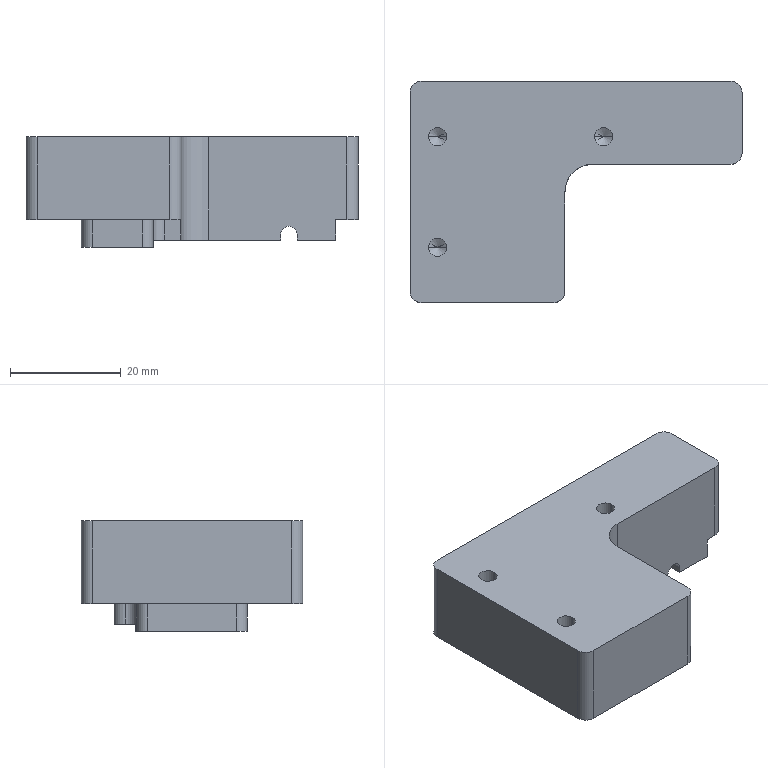Part | STEP file | 05-07 pre-press block | 1 solid | 48 faces | box 60 x 40 x 20 mm | volume 26248 mm3 | cylinder 21 | plane 21 | cone 6 | commonest cylinder face diameters 4 x12 3.3 x6 3 x2 10 x1
STEP:
#1=CARTESIAN_POINT('',(27.5,5.,3.8));
#2=VERTEX_POINT('',#1);
#3=CARTESIAN_POINT('',(29.,5.,2.3));
#4=VERTEX_POINT('',#3);
#5=CARTESIAN_POINT('',(27.5,5.,2.3));
#6=DIRECTION('',(0.,1.,0.));
#7=DIRECTION('',(-1.,0.,0.));
#8=AXIS2_PLACEMENT_3D('',#5,#6,#7);
#9=CIRCLE('',#8,1.5);
#10=EDGE_CURVE('',#2,#4,#9,.T.);
#11=ORIENTED_EDGE('',*,*,#10,.F.);
#12=CARTESIAN_POINT('',(27.5,14.096,3.8));
#13=VERTEX_POINT('',#12);
#14=CARTESIAN_POINT('',(27.5,4.096,3.8));
#15=DIRECTION('',(0.,1.,0.));
#16=VECTOR('',#15,1000.);
#17=LINE('',#14,#16);
#18=EDGE_CURVE('',#2,#13,#17,.T.);
#19=ORIENTED_EDGE('',*,*,#18,.T.);
#20=CARTESIAN_POINT('',(29.,14.096,2.3));
#21=VERTEX_POINT('',#20);
#22=CARTESIAN_POINT('',(27.5,14.096,2.3));
#23=DIRECTION('',(0.,1.,0.));
#24=DIRECTION('',(0.,0.,1.));
#25=AXIS2_PLACEMENT_3D('',#22,#23,#24);
#26=CIRCLE('',#25,1.5);
#27=EDGE_CURVE('',#13,#21,#26,.T.);
#28=ORIENTED_EDGE('',*,*,#27,.T.);
#29=CARTESIAN_POINT('',(29.,4.096,2.3));
#30=DIRECTION('',(0.,1.,0.));
#31=VECTOR('',#30,1000.);
#32=LINE('',#29,#31);
#33=EDGE_CURVE('',#4,#21,#32,.T.);
#34=ORIENTED_EDGE('',*,*,#33,.F.);
#35=EDGE_LOOP('',(#11,#19,#28,#34));
#36=FACE_OUTER_BOUND('',#35,.T.);
#37=CARTESIAN_POINT('',(27.5,4.096,2.3));
#38=DIRECTION('',(0.,1.,0.));
#39=DIRECTION('',(0.,0.,1.));
#40=AXIS2_PLACEMENT_3D('',#37,#38,#39);
#41=CYLINDRICAL_SURFACE('',#40,1.5);
#42=ADVANCED_FACE('',(#36),#41,.F.);
#43=CARTESIAN_POINT('',(-16.65,-10.,8.5));
#44=VERTEX_POINT('',#43);
#45=CARTESIAN_POINT('',(-13.35,-10.,8.5));
#46=VERTEX_POINT('',#45);
#47=CARTESIAN_POINT('',(-15.,-10.,8.5));
#48=DIRECTION('',(0.,0.,1.));
#49=DIRECTION('',(1.,0.,0.));
#50=AXIS2_PLACEMENT_3D('',#47,#48,#49);
#51=CIRCLE('',#50,1.65);
#52=EDGE_CURVE('',#44,#46,#51,.T.);
#53=ORIENTED_EDGE('',*,*,#52,.F.);
#54=CARTESIAN_POINT('',(-16.65,-10.,20.));
#55=VERTEX_POINT('',#54);
#56=CARTESIAN_POINT('',(-16.65,-10.,20.));
#57=DIRECTION('',(0.,0.,1.));
#58=VECTOR('',#57,1000.);
#59=LINE('',#56,#58);
#60=EDGE_CURVE('',#44,#55,#59,.T.);
#61=ORIENTED_EDGE('',*,*,#60,.T.);
#62=CARTESIAN_POINT('',(-13.35,-10.,20.));
#63=VERTEX_POINT('',#62);
#64=CARTESIAN_POINT('',(-15.,-10.,20.));
#65=DIRECTION('',(0.,0.,1.));
#66=DIRECTION('',(1.,0.,0.));
#67=AXIS2_PLACEMENT_3D('',#64,#65,#66);
#68=CIRCLE('',#67,1.65);
#69=EDGE_CURVE('',#55,#63,#68,.T.);
#70=ORIENTED_EDGE('',*,*,#69,.T.);
#71=CARTESIAN_POINT('',(-13.35,-10.,20.));
#72=DIRECTION('',(0.,0.,1.));
#73=VECTOR('',#72,1000.);
#74=LINE('',#71,#73);
#75=EDGE_CURVE('',#46,#63,#74,.T.);
#76=ORIENTED_EDGE('',*,*,#75,.F.);
#77=EDGE_LOOP('',(#53,#61,#70,#76));
#78=FACE_OUTER_BOUND('',#77,.T.);
#79=CARTESIAN_POINT('',(-15.,-10.,20.));
#80=DIRECTION('',(0.,0.,1.));
#81=DIRECTION('',(1.,0.,0.));
#82=AXIS2_PLACEMENT_3D('',#79,#80,#81);
#83=CYLINDRICAL_SURFACE('',#82,1.65);
#84=ADVANCED_FACE('',(#78),#83,.F.);
#85=CARTESIAN_POINT('',(-15.,-10.,7.509));
#86=VERTEX_POINT('',#85);
#87=CARTESIAN_POINT('',(-13.35,-10.,8.5));
#88=DIRECTION('',(0.8572,0.,0.515));
#89=VECTOR('',#88,1000.);
#90=LINE('',#87,#89);
#91=EDGE_CURVE('',#86,#46,#90,.T.);
#92=ORIENTED_EDGE('',*,*,#91,.F.);
#93=CARTESIAN_POINT('',(-16.65,-10.,8.5));
#94=DIRECTION('',(-0.8572,0.,0.515));
#95=VECTOR('',#94,1000.);
#96=LINE('',#93,#95);
#97=EDGE_CURVE('',#86,#44,#96,.T.);
#98=ORIENTED_EDGE('',*,*,#97,.T.);
#99=ORIENTED_EDGE('',*,*,#52,.T.);
#100=EDGE_LOOP('',(#92,#98,#99));
#101=FACE_OUTER_BOUND('',#100,.T.);
#102=CARTESIAN_POINT('',(-15.,-10.,8.5));
#103=DIRECTION('',(0.,0.,1.));
#104=DIRECTION('',(1.,0.,0.));
#105=AXIS2_PLACEMENT_3D('',#102,#103,#104);
#106=CONICAL_SURFACE('',#105,1.65,1.03);
#107=ADVANCED_FACE('',(#101),#106,.F.);
#108=CARTESIAN_POINT('',(13.35,10.,8.5));
#109=VERTEX_POINT('',#108);
#110=CARTESIAN_POINT('',(16.65,10.,8.5));
#111=VERTEX_POINT('',#110);
#112=CARTESIAN_POINT('',(15.,10.,8.5));
#113=DIRECTION('',(0.,0.,1.));
#114=DIRECTION('',(1.,0.,0.));
#115=AXIS2_PLACEMENT_3D('',#112,#113,#114);
#116=CIRCLE('',#115,1.65);
#117=EDGE_CURVE('',#109,#111,#116,.T.);
#118=ORIENTED_EDGE('',*,*,#117,.F.);
#119=CARTESIAN_POINT('',(13.35,10.,20.));
#120=VERTEX_POINT('',#119);
#121=CARTESIAN_POINT('',(13.35,10.,20.));
#122=DIRECTION('',(0.,0.,1.));
#123=VECTOR('',#122,1000.);
#124=LINE('',#121,#123);
#125=EDGE_CURVE('',#109,#120,#124,.T.);
#126=ORIENTED_EDGE('',*,*,#125,.T.);
#127=CARTESIAN_POINT('',(16.65,10.,20.));
#128=VERTEX_POINT('',#127);
#129=CARTESIAN_POINT('',(15.,10.,20.));
#130=DIRECTION('',(0.,0.,1.));
#131=DIRECTION('',(1.,0.,0.));
#132=AXIS2_PLACEMENT_3D('',#129,#130,#131);
#133=CIRCLE('',#132,1.65);
#134=EDGE_CURVE('',#120,#128,#133,.T.);
#135=ORIENTED_EDGE('',*,*,#134,.T.);
#136=CARTESIAN_POINT('',(16.65,10.,20.));
#137=DIRECTION('',(0.,0.,1.));
#138=VECTOR('',#137,1000.);
#139=LINE('',#136,#138);
#140=EDGE_CURVE('',#111,#128,#139,.T.);
#141=ORIENTED_EDGE('',*,*,#140,.F.);
#142=EDGE_LOOP('',(#118,#126,#135,#141));
#143=FACE_OUTER_BOUND('',#142,.T.);
#144=CARTESIAN_POINT('',(15.,10.,20.));
#145=DIRECTION('',(0.,0.,1.));
#146=DIRECTION('',(1.,0.,0.));
#147=AXIS2_PLACEMENT_3D('',#144,#145,#146);
#148=CYLINDRICAL_SURFACE('',#147,1.65);
#149=ADVANCED_FACE('',(#143),#148,.F.);
#150=CARTESIAN_POINT('',(15.,10.,7.509));
#151=VERTEX_POINT('',#150);
#152=CARTESIAN_POINT('',(16.65,10.,8.5));
#153=DIRECTION('',(0.8572,0.,0.515));
#154=VECTOR('',#153,1000.);
#155=LINE('',#152,#154);
#156=EDGE_CURVE('',#151,#111,#155,.T.);
#157=ORIENTED_EDGE('',*,*,#156,.F.);
#158=CARTESIAN_POINT('',(13.35,10.,8.5));
#159=DIRECTION('',(-0.8572,0.,0.515));
#160=VECTOR('',#159,1000.);
#161=LINE('',#158,#160);
#162=EDGE_CURVE('',#151,#109,#161,.T.);
#163=ORIENTED_EDGE('',*,*,#162,.T.);
#164=ORIENTED_EDGE('',*,*,#117,.T.);
#165=EDGE_LOOP('',(#157,#163,#164));
#166=FACE_OUTER_BOUND('',#165,.T.);
#167=CARTESIAN_POINT('',(15.,10.,8.5));
#168=DIRECTION('',(0.,0.,1.));
#169=DIRECTION('',(1.,0.,0.));
#170=AXIS2_PLACEMENT_3D('',#167,#168,#169);
#171=CONICAL_SURFACE('',#170,1.65,1.03);
#172=ADVANCED_FACE('',(#166),#171,.F.);
#173=CARTESIAN_POINT('',(-16.65,10.,8.5));
#174=VERTEX_POINT('',#173);
#175=CARTESIAN_POINT('',(-13.35,10.,8.5));
#176=VERTEX_POINT('',#175);
#177=CARTESIAN_POINT('',(-15.,10.,8.5));
#178=DIRECTION('',(0.,0.,1.));
#179=DIRECTION('',(1.,0.,0.));
#180=AXIS2_PLACEMENT_3D('',#177,#178,#179);
#181=CIRCLE('',#180,1.65);
#182=EDGE_CURVE('',#174,#176,#181,.T.);
#183=ORIENTED_EDGE('',*,*,#182,.F.);
#184=CARTESIAN_POINT('',(-16.65,10.,20.));
#185=VERTEX_POINT('',#184);
#186=CARTESIAN_POINT('',(-16.65,10.,20.));
#187=DIRECTION('',(0.,0.,1.));
#188=VECTOR('',#187,1000.);
#189=LINE('',#186,#188);
#190=EDGE_CURVE('',#174,#185,#189,.T.);
#191=ORIENTED_EDGE('',*,*,#190,.T.);
#192=CARTESIAN_POINT('',(-13.35,10.,20.));
#193=VERTEX_POINT('',#192);
#194=CARTESIAN_POINT('',(-15.,10.,20.));
#195=DIRECTION('',(0.,0.,1.));
#196=DIRECTION('',(1.,0.,0.));
#197=AXIS2_PLACEMENT_3D('',#194,#195,#196);
#198=CIRCLE('',#197,1.65);
#199=EDGE_CURVE('',#185,#193,#198,.T.);
#200=ORIENTED_EDGE('',*,*,#199,.T.);
#201=CARTESIAN_POINT('',(-13.35,10.,20.));
#202=DIRECTION('',(0.,0.,1.));
#203=VECTOR('',#202,1000.);
#204=LINE('',#201,#203);
#205=EDGE_CURVE('',#176,#193,#204,.T.);
#206=ORIENTED_EDGE('',*,*,#205,.F.);
#207=EDGE_LOOP('',(#183,#191,#200,#206));
#208=FACE_OUTER_BOUND('',#207,.T.);
#209=CARTESIAN_POINT('',(-15.,10.,20.));
#210=DIRECTION('',(0.,0.,1.));
#211=DIRECTION('',(1.,0.,0.));
#212=AXIS2_PLACEMENT_3D('',#209,#210,#211);
#213=CYLINDRICAL_SURFACE('',#212,1.65);
#214=ADVANCED_FACE('',(#208),#213,.F.);
#215=CARTESIAN_POINT('',(-15.,10.,7.509));
#216=VERTEX_POINT('',#215);
#217=CARTESIAN_POINT('',(-13.35,10.,8.5));
#218=DIRECTION('',(0.8572,0.,0.515));
#219=VECTOR('',#218,1000.);
#220=LINE('',#217,#219);
#221=EDGE_CURVE('',#216,#176,#220,.T.);
#222=ORIENTED_EDGE('',*,*,#221,.F.);
#223=CARTESIAN_POINT('',(-16.65,10.,8.5));
#224=DIRECTION('',(-0.8572,0.,0.515));
#225=VECTOR('',#224,1000.);
#226=LINE('',#223,#225);
#227=EDGE_CURVE('',#216,#174,#226,.T.);
#228=ORIENTED_EDGE('',*,*,#227,.T.);
#229=ORIENTED_EDGE('',*,*,#182,.T.);
#230=EDGE_LOOP('',(#222,#228,#229));
#231=FACE_OUTER_BOUND('',#230,.T.);
#232=CARTESIAN_POINT('',(-15.,10.,8.5));
#233=DIRECTION('',(0.,0.,1.));
#234=DIRECTION('',(1.,0.,0.));
#235=AXIS2_PLACEMENT_3D('',#232,#233,#234);
#236=CONICAL_SURFACE('',#235,1.65,1.03);
#237=ADVANCED_FACE('',(#231),#236,.F.);
#238=CARTESIAN_POINT('',(6.093,14.096,1.3));
#239=VERTEX_POINT('',#238);
#240=CARTESIAN_POINT('',(26.,14.096,1.3));
#241=VERTEX_POINT('',#240);
#242=CARTESIAN_POINT('',(20.,14.096,1.3));
#243=DIRECTION('',(1.,0.,0.));
#244=VECTOR('',#243,1000.);
#245=LINE('',#242,#244);
#246=EDGE_CURVE('',#239,#241,#245,.T.);
#247=ORIENTED_EDGE('',*,*,#246,.T.);
#248=CARTESIAN_POINT('',(26.,5.,1.3));
#249=VERTEX_POINT('',#248);
#250=CARTESIAN_POINT('',(26.,4.096,1.3));
#251=DIRECTION('',(0.,1.,0.));
#252=VECTOR('',#251,1000.);
#253=LINE('',#250,#252);
#254=EDGE_CURVE('',#249,#241,#253,.T.);
#255=ORIENTED_EDGE('',*,*,#254,.F.);
#256=CARTESIAN_POINT('',(13.,5.,1.3));
#257=VERTEX_POINT('',#256);
#258=CARTESIAN_POINT('',(20.,5.,1.3));
#259=DIRECTION('',(-1.,0.,0.));
#260=VECTOR('',#259,1000.);
#261=LINE('',#258,#260);
#262=EDGE_CURVE('',#249,#257,#261,.T.);
#263=ORIENTED_EDGE('',*,*,#262,.T.);
#264=CARTESIAN_POINT('',(8.,0.,1.3));
#265=VERTEX_POINT('',#264);
#266=CARTESIAN_POINT('',(13.,0.,1.3));
#267=DIRECTION('',(0.,0.,1.));
#268=DIRECTION('',(1.,0.,0.));
#269=AXIS2_PLACEMENT_3D('',#266,#267,#268);
#270=CIRCLE('',#269,5.);
#271=EDGE_CURVE('',#257,#265,#270,.T.);
#272=ORIENTED_EDGE('',*,*,#271,.T.);
#273=CARTESIAN_POINT('',(8.,-5.5,1.3));
#274=VERTEX_POINT('',#273);
#275=CARTESIAN_POINT('',(8.,26.,1.3));
#276=DIRECTION('',(0.,-1.,0.));
#277=VECTOR('',#276,1000.);
#278=LINE('',#275,#277);
#279=EDGE_CURVE('',#265,#274,#278,.T.);
#280=ORIENTED_EDGE('',*,*,#279,.T.);
#281=CARTESIAN_POINT('',(5.,-5.5,1.3));
#282=VERTEX_POINT('',#281);
#283=CARTESIAN_POINT('',(20.,-5.5,1.3));
#284=DIRECTION('',(-1.,0.,0.));
#285=VECTOR('',#284,1000.);
#286=LINE('',#283,#285);
#287=EDGE_CURVE('',#274,#282,#286,.T.);
#288=ORIENTED_EDGE('',*,*,#287,.T.);
#289=CARTESIAN_POINT('',(3.,-7.5,1.3));
#290=VERTEX_POINT('',#289);
#291=CARTESIAN_POINT('',(5.,-7.5,1.3));
#292=DIRECTION('',(0.,0.,1.));
#293=DIRECTION('',(1.,0.,0.));
#294=AXIS2_PLACEMENT_3D('',#291,#292,#293);
#295=CIRCLE('',#294,2.);
#296=EDGE_CURVE('',#282,#290,#295,.T.);
#297=ORIENTED_EDGE('',*,*,#296,.T.);
#298=CARTESIAN_POINT('',(3.,10.218,1.3));
#299=VERTEX_POINT('',#298);
#300=CARTESIAN_POINT('',(3.,26.,1.3));
#301=DIRECTION('',(0.,-1.,0.));
#302=VECTOR('',#301,1000.);
#303=LINE('',#300,#302);
#304=EDGE_CURVE('',#299,#290,#303,.T.);
#305=ORIENTED_EDGE('',*,*,#304,.F.);
#306=CARTESIAN_POINT('',(4.093,12.,1.3));
#307=VERTEX_POINT('',#306);
#308=CARTESIAN_POINT('',(2.093,12.,1.3));
#309=DIRECTION('',(0.,0.,1.));
#310=DIRECTION('',(1.,0.,0.));
#311=AXIS2_PLACEMENT_3D('',#308,#309,#310);
#312=CIRCLE('',#311,2.);
#313=EDGE_CURVE('',#299,#307,#312,.T.);
#314=ORIENTED_EDGE('',*,*,#313,.T.);
#315=CARTESIAN_POINT('',(4.093,12.096,1.3));
#316=VERTEX_POINT('',#315);
#317=CARTESIAN_POINT('',(4.093,26.,1.3));
#318=DIRECTION('',(0.,1.,0.));
#319=VECTOR('',#318,1000.);
#320=LINE('',#317,#319);
#321=EDGE_CURVE('',#307,#316,#320,.T.);
#322=ORIENTED_EDGE('',*,*,#321,.T.);
#323=CARTESIAN_POINT('',(6.093,12.096,1.3));
#324=DIRECTION('',(0.,0.,-1.));
#325=DIRECTION('',(1.,0.,0.));
#326=AXIS2_PLACEMENT_3D('',#323,#324,#325);
#327=CIRCLE('',#326,2.);
#328=EDGE_CURVE('',#316,#239,#327,.T.);
#329=ORIENTED_EDGE('',*,*,#328,.T.);
#330=EDGE_LOOP('',(#247,#255,#263,#272,#280,#288,#297,#305,#314,#322,#329));
#331=FACE_OUTER_BOUND('',#330,.T.);
#332=CARTESIAN_POINT('',(20.,26.,1.3));
#333=DIRECTION('',(0.,0.,1.));
#334=DIRECTION('',(1.,0.,0.));
#335=AXIS2_PLACEMENT_3D('',#332,#333,#334);
#336=PLANE('',#335);
#337=ADVANCED_FACE('',(#331),#336,.F.);
#338=CARTESIAN_POINT('',(38.,5.,5.));
#339=VERTEX_POINT('',#338);
#340=CARTESIAN_POINT('',(36.,5.,5.));
#341=VERTEX_POINT('',#340);
#342=CARTESIAN_POINT('',(18.,5.,5.));
#343=DIRECTION('',(-1.,0.,0.));
#344=VECTOR('',#343,1000.);
#345=LINE('',#342,#344);
#346=EDGE_CURVE('',#339,#341,#345,.T.);
#347=ORIENTED_EDGE('',*,*,#346,.T.);
#348=CARTESIAN_POINT('',(36.,12.096,5.));
#349=VERTEX_POINT('',#348);
#350=CARTESIAN_POINT('',(36.,12.096,5.));
#351=DIRECTION('',(0.,-1.,0.));
#352=VECTOR('',#351,1000.);
#353=LINE('',#350,#352);
#354=EDGE_CURVE('',#349,#341,#353,.T.);
#355=ORIENTED_EDGE('',*,*,#354,.F.);
#356=CARTESIAN_POINT('',(34.,14.096,5.));
#357=VERTEX_POINT('',#356);
#358=CARTESIAN_POINT('',(34.,12.096,5.));
#359=DIRECTION('',(0.,0.,-1.));
#360=DIRECTION('',(1.,0.,0.));
#361=AXIS2_PLACEMENT_3D('',#358,#359,#360);
#362=CIRCLE('',#361,2.);
#363=EDGE_CURVE('',#357,#349,#362,.T.);
#364=ORIENTED_EDGE('',*,*,#363,.F.);
#365=CARTESIAN_POINT('',(6.093,14.096,5.));
#366=VERTEX_POINT('',#365);
#367=CARTESIAN_POINT('',(20.,14.096,5.));
#368=DIRECTION('',(-1.,0.,0.));
#369=VECTOR('',#368,1000.);
#370=LINE('',#367,#369);
#371=EDGE_CURVE('',#357,#366,#370,.T.);
#372=ORIENTED_EDGE('',*,*,#371,.T.);
#373=CARTESIAN_POINT('',(4.093,12.096,5.));
#374=VERTEX_POINT('',#373);
#375=CARTESIAN_POINT('',(6.093,12.096,5.));
#376=DIRECTION('',(0.,0.,1.));
#377=DIRECTION('',(-1.,0.,0.));
#378=AXIS2_PLACEMENT_3D('',#375,#376,#377);
#379=CIRCLE('',#378,2.);
#380=EDGE_CURVE('',#366,#374,#379,.T.);
#381=ORIENTED_EDGE('',*,*,#380,.T.);
#382=CARTESIAN_POINT('',(4.093,12.,5.));
#383=VERTEX_POINT('',#382);
#384=CARTESIAN_POINT('',(4.093,14.096,5.));
#385=DIRECTION('',(0.,-1.,0.));
#386=VECTOR('',#385,1000.);
#387=LINE('',#384,#386);
#388=EDGE_CURVE('',#374,#383,#387,.T.);
#389=ORIENTED_EDGE('',*,*,#388,.T.);
#390=CARTESIAN_POINT('',(2.093,10.,5.));
#391=VERTEX_POINT('',#390);
#392=CARTESIAN_POINT('',(2.093,12.,5.));
#393=DIRECTION('',(0.,0.,-1.));
#394=DIRECTION('',(-1.,0.,0.));
#395=AXIS2_PLACEMENT_3D('',#392,#393,#394);
#396=CIRCLE('',#395,2.);
#397=EDGE_CURVE('',#383,#391,#396,.T.);
#398=ORIENTED_EDGE('',*,*,#397,.T.);
#399=CARTESIAN_POINT('',(-8.,10.,5.));
#400=VERTEX_POINT('',#399);
#401=CARTESIAN_POINT('',(4.093,10.,5.));
#402=DIRECTION('',(-1.,0.,0.));
#403=VECTOR('',#402,1000.);
#404=LINE('',#401,#403);
#405=EDGE_CURVE('',#391,#400,#404,.T.);
#406=ORIENTED_EDGE('',*,*,#405,.T.);
#407=CARTESIAN_POINT('',(-10.,8.,5.));
#408=VERTEX_POINT('',#407);
#409=CARTESIAN_POINT('',(-8.,8.,5.));
#410=DIRECTION('',(0.,0.,1.));
#411=DIRECTION('',(-1.,0.,0.));
#412=AXIS2_PLACEMENT_3D('',#409,#410,#411);
#413=CIRCLE('',#412,2.);
#414=EDGE_CURVE('',#400,#408,#413,.T.);
#415=ORIENTED_EDGE('',*,*,#414,.T.);
#416=CARTESIAN_POINT('',(-10.,-8.,5.));
#417=VERTEX_POINT('',#416);
#418=CARTESIAN_POINT('',(-10.,10.,5.));
#419=DIRECTION('',(0.,-1.,0.));
#420=VECTOR('',#419,1000.);
#421=LINE('',#418,#420);
#422=EDGE_CURVE('',#408,#417,#421,.T.);
#423=ORIENTED_EDGE('',*,*,#422,.T.);
#424=CARTESIAN_POINT('',(-8.,-10.,5.));
#425=VERTEX_POINT('',#424);
#426=CARTESIAN_POINT('',(-8.,-8.,5.));
#427=DIRECTION('',(0.,0.,1.));
#428=DIRECTION('',(-1.,0.,0.));
#429=AXIS2_PLACEMENT_3D('',#426,#427,#428);
#430=CIRCLE('',#429,2.);
#431=EDGE_CURVE('',#417,#425,#430,.T.);
#432=ORIENTED_EDGE('',*,*,#431,.T.);
#433=CARTESIAN_POINT('',(1.,-10.,5.));
#434=VERTEX_POINT('',#433);
#435=CARTESIAN_POINT('',(3.,-10.,5.));
#436=DIRECTION('',(1.,0.,0.));
#437=VECTOR('',#436,1000.);
#438=LINE('',#435,#437);
#439=EDGE_CURVE('',#425,#434,#438,.T.);
#440=ORIENTED_EDGE('',*,*,#439,.T.);
#441=CARTESIAN_POINT('',(3.,-8.,5.));
#442=VERTEX_POINT('',#441);
#443=CARTESIAN_POINT('',(1.,-8.,5.));
#444=DIRECTION('',(0.,0.,1.));
#445=DIRECTION('',(-1.,0.,0.));
#446=AXIS2_PLACEMENT_3D('',#443,#444,#445);
#447=CIRCLE('',#446,2.);
#448=EDGE_CURVE('',#434,#442,#447,.T.);
#449=ORIENTED_EDGE('',*,*,#448,.T.);
#450=CARTESIAN_POINT('',(3.,-7.5,5.));
#451=VERTEX_POINT('',#450);
#452=CARTESIAN_POINT('',(3.,-5.5,5.));
#453=DIRECTION('',(0.,1.,0.));
#454=VECTOR('',#453,1000.);
#455=LINE('',#452,#454);
#456=EDGE_CURVE('',#442,#451,#455,.T.);
#457=ORIENTED_EDGE('',*,*,#456,.T.);
#458=CARTESIAN_POINT('',(5.,-5.5,5.));
#459=VERTEX_POINT('',#458);
#460=CARTESIAN_POINT('',(5.,-7.5,5.));
#461=DIRECTION('',(0.,0.,-1.));
#462=DIRECTION('',(-1.,0.,0.));
#463=AXIS2_PLACEMENT_3D('',#460,#461,#462);
#464=CIRCLE('',#463,2.);
#465=EDGE_CURVE('',#451,#459,#464,.T.);
#466=ORIENTED_EDGE('',*,*,#465,.T.);
#467=CARTESIAN_POINT('',(8.,-5.5,5.));
#468=VERTEX_POINT('',#467);
#469=CARTESIAN_POINT('',(20.,-5.5,5.));
#470=DIRECTION('',(1.,0.,0.));
#471=VECTOR('',#470,1000.);
#472=LINE('',#469,#471);
#473=EDGE_CURVE('',#459,#468,#472,.T.);
#474=ORIENTED_EDGE('',*,*,#473,.T.);
#475=CARTESIAN_POINT('',(8.,-18.,5.));
#476=VERTEX_POINT('',#475);
#477=CARTESIAN_POINT('',(8.,10.,5.));
#478=DIRECTION('',(0.,1.,0.));
#479=VECTOR('',#478,1000.);
#480=LINE('',#477,#479);
#481=EDGE_CURVE('',#476,#468,#480,.T.);
#482=ORIENTED_EDGE('',*,*,#481,.F.);
#483=CARTESIAN_POINT('',(6.,-20.,5.));
#484=VERTEX_POINT('',#483);
#485=CARTESIAN_POINT('',(6.,-18.,5.));
#486=DIRECTION('',(0.,0.,-1.));
#487=DIRECTION('',(-1.,0.,0.));
#488=AXIS2_PLACEMENT_3D('',#485,#486,#487);
#489=CIRCLE('',#488,2.);
#490=EDGE_CURVE('',#476,#484,#489,.T.);
#491=ORIENTED_EDGE('',*,*,#490,.T.);
#492=CARTESIAN_POINT('',(-18.,-20.,5.));
#493=VERTEX_POINT('',#492);
#494=CARTESIAN_POINT('',(-20.,-20.,5.));
#495=DIRECTION('',(-1.,0.,0.));
#496=VECTOR('',#495,1000.);
#497=LINE('',#494,#496);
#498=EDGE_CURVE('',#484,#493,#497,.T.);
#499=ORIENTED_EDGE('',*,*,#498,.T.);
#500=CARTESIAN_POINT('',(-20.,-18.,5.));
#501=VERTEX_POINT('',#500);
#502=CARTESIAN_POINT('',(-18.,-18.,5.));
#503=DIRECTION('',(0.,0.,-1.));
#504=DIRECTION('',(-1.,0.,0.));
#505=AXIS2_PLACEMENT_3D('',#502,#503,#504);
#506=CIRCLE('',#505,2.);
#507=EDGE_CURVE('',#493,#501,#506,.T.);
#508=ORIENTED_EDGE('',*,*,#507,.T.);
#509=CARTESIAN_POINT('',(-20.,18.,5.));
#510=VERTEX_POINT('',#509);
#511=CARTESIAN_POINT('',(-20.,20.,5.));
#512=DIRECTION('',(0.,1.,0.));
#513=VECTOR('',#512,1000.);
#514=LINE('',#511,#513);
#515=EDGE_CURVE('',#501,#510,#514,.T.);
#516=ORIENTED_EDGE('',*,*,#515,.T.);
#517=CARTESIAN_POINT('',(-18.,20.,5.));
#518=VERTEX_POINT('',#517);
#519=CARTESIAN_POINT('',(-18.,18.,5.));
#520=DIRECTION('',(0.,0.,-1.));
#521=DIRECTION('',(-1.,0.,0.));
#522=AXIS2_PLACEMENT_3D('',#519,#520,#521);
#523=CIRCLE('',#522,2.);
#524=EDGE_CURVE('',#510,#518,#523,.T.);
#525=ORIENTED_EDGE('',*,*,#524,.T.);
#526=CARTESIAN_POINT('',(38.,20.,5.));
#527=VERTEX_POINT('',#526);
#528=CARTESIAN_POINT('',(-20.,20.,5.));
#529=DIRECTION('',(1.,0.,0.));
#530=VECTOR('',#529,1000.);
#531=LINE('',#528,#530);
#532=EDGE_CURVE('',#518,#527,#531,.T.);
#533=ORIENTED_EDGE('',*,*,#532,.T.);
#534=CARTESIAN_POINT('',(40.,18.,5.));
#535=VERTEX_POINT('',#534);
#536=CARTESIAN_POINT('',(38.,18.,5.));
#537=DIRECTION('',(0.,0.,-1.));
#538=DIRECTION('',(-1.,0.,0.));
#539=AXIS2_PLACEMENT_3D('',#536,#537,#538);
#540=CIRCLE('',#539,2.);
#541=EDGE_CURVE('',#527,#535,#540,.T.);
#542=ORIENTED_EDGE('',*,*,#541,.T.);
#543=CARTESIAN_POINT('',(40.,7.,5.));
#544=VERTEX_POINT('',#543);
#545=CARTESIAN_POINT('',(40.,20.,5.));
#546=DIRECTION('',(0.,-1.,0.));
#547=VECTOR('',#546,1000.);
#548=LINE('',#545,#547);
#549=EDGE_CURVE('',#535,#544,#548,.T.);
#550=ORIENTED_EDGE('',*,*,#549,.T.);
#551=CARTESIAN_POINT('',(38.,7.,5.));
#552=DIRECTION('',(0.,0.,-1.));
#553=DIRECTION('',(-1.,0.,0.));
#554=AXIS2_PLACEMENT_3D('',#551,#552,#553);
#555=CIRCLE('',#554,2.);
#556=EDGE_CURVE('',#544,#339,#555,.T.);
#557=ORIENTED_EDGE('',*,*,#556,.T.);
#558=EDGE_LOOP('',(#347,#355,#364,#372,#381,#389,#398,#406,#415,#423,#432,#440,#449,#457,#466,#474,#482,#491,#499,#508,#516,#525,#533,#542,#550,#557));
#559=FACE_OUTER_BOUND('',#558,.T.);
#560=CARTESIAN_POINT('',(4.093,10.,5.));
#561=DIRECTION('',(0.,0.,-1.));
#562=DIRECTION('',(-1.,0.,0.));
#563=AXIS2_PLACEMENT_3D('',#560,#561,#562);
#564=PLANE('',#563);
#565=ADVANCED_FACE('',(#559),#564,.T.);
#566=CARTESIAN_POINT('',(38.,20.,20.));
#567=VERTEX_POINT('',#566);
#568=CARTESIAN_POINT('',(-18.,20.,20.));
#569=VERTEX_POINT('',#568);
#570=CARTESIAN_POINT('',(-20.,20.,20.));
#571=DIRECTION('',(-1.,0.,0.));
#572=VECTOR('',#571,1000.);
#573=LINE('',#570,#572);
#574=EDGE_CURVE('',#567,#569,#573,.T.);
#575=ORIENTED_EDGE('',*,*,#574,.F.);
#576=CARTESIAN_POINT('',(38.,20.,5.));
#577=DIRECTION('',(0.,0.,-1.));
#578=VECTOR('',#577,1000.);
#579=LINE('',#576,#578);
#580=EDGE_CURVE('',#567,#527,#579,.T.);
#581=ORIENTED_EDGE('',*,*,#580,.T.);
#582=ORIENTED_EDGE('',*,*,#532,.F.);
#583=CARTESIAN_POINT('',(-18.,20.,20.));
#584=DIRECTION('',(0.,0.,1.));
#585=VECTOR('',#584,1000.);
#586=LINE('',#583,#585);
#587=EDGE_CURVE('',#518,#569,#586,.T.);
#588=ORIENTED_EDGE('',*,*,#587,.T.);
#589=EDGE_LOOP('',(#575,#581,#582,#588));
#590=FACE_OUTER_BOUND('',#589,.T.);
#591=CARTESIAN_POINT('',(-20.,20.,20.));
#592=DIRECTION('',(0.,-1.,0.));
#593=DIRECTION('',(0.,0.,-1.));
#594=AXIS2_PLACEMENT_3D('',#591,#592,#593);
#595=PLANE('',#594);
#596=ADVANCED_FACE('',(#590),#595,.F.);
#597=CARTESIAN_POINT('',(-20.,18.,20.));
#598=VERTEX_POINT('',#597);
#599=CARTESIAN_POINT('',(-20.,-18.,20.));
#600=VERTEX_POINT('',#599);
#601=CARTESIAN_POINT('',(-20.,20.,20.));
#602=DIRECTION('',(0.,-1.,0.));
#603=VECTOR('',#602,1000.);
#604=LINE('',#601,#603);
#605=EDGE_CURVE('',#598,#600,#604,.T.);
#606=ORIENTED_EDGE('',*,*,#605,.F.);
#607=CARTESIAN_POINT('',(-20.,18.,20.));
#608=DIRECTION('',(0.,0.,-1.));
#609=VECTOR('',#608,1000.);
#610=LINE('',#607,#609);
#611=EDGE_CURVE('',#598,#510,#610,.T.);
#612=ORIENTED_EDGE('',*,*,#611,.T.);
#613=ORIENTED_EDGE('',*,*,#515,.F.);
#614=CARTESIAN_POINT('',(-20.,-18.,20.));
#615=DIRECTION('',(0.,0.,1.));
#616=VECTOR('',#615,1000.);
#617=LINE('',#614,#616);
#618=EDGE_CURVE('',#501,#600,#617,.T.);
#619=ORIENTED_EDGE('',*,*,#618,.T.);
#620=EDGE_LOOP('',(#606,#612,#613,#619));
#621=FACE_OUTER_BOUND('',#620,.T.);
#622=CARTESIAN_POINT('',(-20.,20.,20.));
#623=DIRECTION('',(1.,0.,0.));
#624=DIRECTION('',(0.,1.,0.));
#625=AXIS2_PLACEMENT_3D('',#622,#623,#624);
#626=PLANE('',#625);
#627=ADVANCED_FACE('',(#621),#626,.F.);
#628=ORIENTED_EDGE('',*,*,#498,.F.);
#629=CARTESIAN_POINT('',(6.,-20.,20.));
#630=VERTEX_POINT('',#629);
#631=CARTESIAN_POINT('',(6.,-20.,20.));
#632=DIRECTION('',(0.,0.,1.));
#633=VECTOR('',#632,1000.);
#634=LINE('',#631,#633);
#635=EDGE_CURVE('',#484,#630,#634,.T.);
#636=ORIENTED_EDGE('',*,*,#635,.T.);
#637=CARTESIAN_POINT('',(-18.,-20.,20.));
#638=VERTEX_POINT('',#637);
#639=CARTESIAN_POINT('',(-20.,-20.,20.));
#640=DIRECTION('',(1.,0.,0.));
#641=VECTOR('',#640,1000.);
#642=LINE('',#639,#641);
#643=EDGE_CURVE('',#638,#630,#642,.T.);
#644=ORIENTED_EDGE('',*,*,#643,.F.);
#645=CARTESIAN_POINT('',(-18.,-20.,20.));
#646=DIRECTION('',(0.,0.,-1.));
#647=VECTOR('',#646,1000.);
#648=LINE('',#645,#647);
#649=EDGE_CURVE('',#638,#493,#648,.T.);
#650=ORIENTED_EDGE('',*,*,#649,.T.);
#651=EDGE_LOOP('',(#628,#636,#644,#650));
#652=FACE_OUTER_BOUND('',#651,.T.);
#653=CARTESIAN_POINT('',(-20.,-20.,20.));
#654=DIRECTION('',(0.,1.,0.));
#655=DIRECTION('',(0.,0.,1.));
#656=AXIS2_PLACEMENT_3D('',#653,#654,#655);
#657=PLANE('',#656);
#658=ADVANCED_FACE('',(#652),#657,.F.);
#659=CARTESIAN_POINT('',(40.,18.,20.));
#660=VERTEX_POINT('',#659);
#661=CARTESIAN_POINT('',(40.,7.,20.));
#662=VERTEX_POINT('',#661);
#663=CARTESIAN_POINT('',(40.,20.,20.));
#664=DIRECTION('',(0.,-1.,0.));
#665=VECTOR('',#664,1000.);
#666=LINE('',#663,#665);
#667=EDGE_CURVE('',#660,#662,#666,.T.);
#668=ORIENTED_EDGE('',*,*,#667,.F.);
#669=CARTESIAN_POINT('',(38.,18.,20.));
#670=DIRECTION('',(0.,0.,1.));
#671=DIRECTION('',(1.,0.,0.));
#672=AXIS2_PLACEMENT_3D('',#669,#670,#671);
#673=CIRCLE('',#672,2.);
#674=EDGE_CURVE('',#660,#567,#673,.T.);
#675=ORIENTED_EDGE('',*,*,#674,.T.);
#676=ORIENTED_EDGE('',*,*,#574,.T.);
#677=CARTESIAN_POINT('',(-18.,18.,20.));
#678=DIRECTION('',(0.,0.,1.));
#679=DIRECTION('',(1.,0.,0.));
#680=AXIS2_PLACEMENT_3D('',#677,#678,#679);
#681=CIRCLE('',#680,2.);
#682=EDGE_CURVE('',#569,#598,#681,.T.);
#683=ORIENTED_EDGE('',*,*,#682,.T.);
#684=ORIENTED_EDGE('',*,*,#605,.T.);
#685=CARTESIAN_POINT('',(-18.,-18.,20.));
#686=DIRECTION('',(0.,0.,1.));
#687=DIRECTION('',(1.,0.,0.));
#688=AXIS2_PLACEMENT_3D('',#685,#686,#687);
#689=CIRCLE('',#688,2.);
#690=EDGE_CURVE('',#600,#638,#689,.T.);
#691=ORIENTED_EDGE('',*,*,#690,.T.);
#692=ORIENTED_EDGE('',*,*,#643,.T.);
#693=CARTESIAN_POINT('',(8.,-18.,20.));
#694=VERTEX_POINT('',#693);
#695=CARTESIAN_POINT('',(6.,-18.,20.));
#696=DIRECTION('',(0.,0.,1.));
#697=DIRECTION('',(1.,0.,0.));
#698=AXIS2_PLACEMENT_3D('',#695,#696,#697);
#699=CIRCLE('',#698,2.);
#700=EDGE_CURVE('',#630,#694,#699,.T.);
#701=ORIENTED_EDGE('',*,*,#700,.T.);
#702=CARTESIAN_POINT('',(8.,0.,20.));
#703=VERTEX_POINT('',#702);
#704=CARTESIAN_POINT('',(8.,0.,20.));
#705=DIRECTION('',(0.,-1.,0.));
#706=VECTOR('',#705,1000.);
#707=LINE('',#704,#706);
#708=EDGE_CURVE('',#703,#694,#707,.T.);
#709=ORIENTED_EDGE('',*,*,#708,.F.);
#710=CARTESIAN_POINT('',(13.,5.,20.));
#711=VERTEX_POINT('',#710);
#712=CARTESIAN_POINT('',(13.,0.,20.));
#713=DIRECTION('',(0.,0.,1.));
#714=DIRECTION('',(-1.,0.,0.));
#715=AXIS2_PLACEMENT_3D('',#712,#713,#714);
#716=CIRCLE('',#715,5.);
#717=EDGE_CURVE('',#711,#703,#716,.T.);
#718=ORIENTED_EDGE('',*,*,#717,.F.);
#719=CARTESIAN_POINT('',(38.,5.,20.));
#720=VERTEX_POINT('',#719);
#721=CARTESIAN_POINT('',(31.615,5.,20.));
#722=DIRECTION('',(-1.,0.,0.));
#723=VECTOR('',#722,1000.);
#724=LINE('',#721,#723);
#725=EDGE_CURVE('',#720,#711,#724,.T.);
#726=ORIENTED_EDGE('',*,*,#725,.F.);
#727=CARTESIAN_POINT('',(38.,7.,20.));
#728=DIRECTION('',(0.,0.,1.));
#729=DIRECTION('',(1.,0.,0.));
#730=AXIS2_PLACEMENT_3D('',#727,#728,#729);
#731=CIRCLE('',#730,2.);
#732=EDGE_CURVE('',#720,#662,#731,.T.);
#733=ORIENTED_EDGE('',*,*,#732,.T.);
#734=EDGE_LOOP('',(#668,#675,#676,#683,#684,#691,#692,#701,#709,#718,#726,#733));
#735=FACE_OUTER_BOUND('',#734,.T.);
#736=CARTESIAN_POINT('',(-15.,-10.,20.));
#737=DIRECTION('',(0.,0.,1.));
#738=DIRECTION('',(1.,0.,0.));
#739=AXIS2_PLACEMENT_3D('',#736,#737,#738);
#740=CIRCLE('',#739,1.65);
#741=EDGE_CURVE('',#63,#55,#740,.T.);
#742=ORIENTED_EDGE('',*,*,#741,.F.);
#743=ORIENTED_EDGE('',*,*,#69,.F.);
#744=EDGE_LOOP('',(#742,#743));
#745=FACE_BOUND('',#744,.T.);
#746=CARTESIAN_POINT('',(15.,10.,20.));
#747=DIRECTION('',(0.,0.,1.));
#748=DIRECTION('',(1.,0.,0.));
#749=AXIS2_PLACEMENT_3D('',#746,#747,#748);
#750=CIRCLE('',#749,1.65);
#751=EDGE_CURVE('',#128,#120,#750,.T.);
#752=ORIENTED_EDGE('',*,*,#751,.F.);
#753=ORIENTED_EDGE('',*,*,#134,.F.);
#754=EDGE_LOOP('',(#752,#753));
#755=FACE_BOUND('',#754,.T.);
#756=CARTESIAN_POINT('',(-15.,10.,20.));
#757=DIRECTION('',(0.,0.,1.));
#758=DIRECTION('',(1.,0.,0.));
#759=AXIS2_PLACEMENT_3D('',#756,#757,#758);
#760=CIRCLE('',#759,1.65);
#761=EDGE_CURVE('',#193,#185,#760,.T.);
#762=ORIENTED_EDGE('',*,*,#761,.F.);
#763=ORIENTED_EDGE('',*,*,#199,.F.);
#764=EDGE_LOOP('',(#762,#763));
#765=FACE_BOUND('',#764,.T.);
#766=CARTESIAN_POINT('',(20.,-20.,20.));
#767=DIRECTION('',(0.,0.,1.));
#768=DIRECTION('',(1.,0.,0.));
#769=AXIS2_PLACEMENT_3D('',#766,#767,#768);
#770=PLANE('',#769);
#771=ADVANCED_FACE('',(#735,#745,#755,#765),#770,.T.);
#772=CARTESIAN_POINT('',(3.,10.218,0.));
#773=VERTEX_POINT('',#772);
#774=CARTESIAN_POINT('',(3.,-8.,0.));
#775=VERTEX_POINT('',#774);
#776=CARTESIAN_POINT('',(3.,-20.,0.));
#777=DIRECTION('',(0.,-1.,0.));
#778=VECTOR('',#777,1000.);
#779=LINE('',#776,#778);
#780=EDGE_CURVE('',#773,#775,#779,.T.);
#781=ORIENTED_EDGE('',*,*,#780,.T.);
#782=CARTESIAN_POINT('',(1.,-10.,0.));
#783=VERTEX_POINT('',#782);
#784=CARTESIAN_POINT('',(1.,-8.,0.));
#785=DIRECTION('',(0.,0.,-1.));
#786=DIRECTION('',(1.,0.,0.));
#787=AXIS2_PLACEMENT_3D('',#784,#785,#786);
#788=CIRCLE('',#787,2.);
#789=EDGE_CURVE('',#775,#783,#788,.T.);
#790=ORIENTED_EDGE('',*,*,#789,.T.);
#791=CARTESIAN_POINT('',(-8.,-10.,0.));
#792=VERTEX_POINT('',#791);
#793=CARTESIAN_POINT('',(3.,-10.,0.));
#794=DIRECTION('',(1.,0.,0.));
#795=VECTOR('',#794,1000.);
#796=LINE('',#793,#795);
#797=EDGE_CURVE('',#792,#783,#796,.T.);
#798=ORIENTED_EDGE('',*,*,#797,.F.);
#799=CARTESIAN_POINT('',(-10.,-8.,0.));
#800=VERTEX_POINT('',#799);
#801=CARTESIAN_POINT('',(-8.,-8.,0.));
#802=DIRECTION('',(0.,0.,-1.));
#803=DIRECTION('',(1.,0.,0.));
#804=AXIS2_PLACEMENT_3D('',#801,#802,#803);
#805=CIRCLE('',#804,2.);
#806=EDGE_CURVE('',#792,#800,#805,.T.);
#807=ORIENTED_EDGE('',*,*,#806,.T.);
#808=CARTESIAN_POINT('',(-10.,8.,0.));
#809=VERTEX_POINT('',#808);
#810=CARTESIAN_POINT('',(-10.,10.,0.));
#811=DIRECTION('',(0.,-1.,0.));
#812=VECTOR('',#811,1000.);
#813=LINE('',#810,#812);
#814=EDGE_CURVE('',#809,#800,#813,.T.);
#815=ORIENTED_EDGE('',*,*,#814,.F.);
#816=CARTESIAN_POINT('',(-8.,10.,0.));
#817=VERTEX_POINT('',#816);
#818=CARTESIAN_POINT('',(-8.,8.,0.));
#819=DIRECTION('',(0.,0.,-1.));
#820=DIRECTION('',(1.,0.,0.));
#821=AXIS2_PLACEMENT_3D('',#818,#819,#820);
#822=CIRCLE('',#821,2.);
#823=EDGE_CURVE('',#809,#817,#822,.T.);
#824=ORIENTED_EDGE('',*,*,#823,.T.);
#825=CARTESIAN_POINT('',(2.093,10.,0.));
#826=VERTEX_POINT('',#825);
#827=CARTESIAN_POINT('',(4.093,10.,0.));
#828=DIRECTION('',(-1.,0.,0.));
#829=VECTOR('',#828,1000.);
#830=LINE('',#827,#829);
#831=EDGE_CURVE('',#826,#817,#830,.T.);
#832=ORIENTED_EDGE('',*,*,#831,.F.);
#833=CARTESIAN_POINT('',(2.093,12.,0.));
#834=DIRECTION('',(0.,0.,1.));
#835=DIRECTION('',(1.,0.,0.));
#836=AXIS2_PLACEMENT_3D('',#833,#834,#835);
#837=CIRCLE('',#836,2.);
#838=EDGE_CURVE('',#826,#773,#837,.T.);
#839=ORIENTED_EDGE('',*,*,#838,.T.);
#840=EDGE_LOOP('',(#781,#790,#798,#807,#815,#824,#832,#839));
#841=FACE_OUTER_BOUND('',#840,.T.);
#842=CARTESIAN_POINT('',(20.,-20.,0.));
#843=DIRECTION('',(0.,0.,1.));
#844=DIRECTION('',(1.,0.,0.));
#845=AXIS2_PLACEMENT_3D('',#842,#843,#844);
#846=PLANE('',#845);
#847=ADVANCED_FACE('',(#841),#846,.F.);
#848=CARTESIAN_POINT('',(36.,5.,1.3));
#849=VERTEX_POINT('',#848);
#850=CARTESIAN_POINT('',(29.,5.,1.3));
#851=VERTEX_POINT('',#850);
#852=CARTESIAN_POINT('',(20.,5.,1.3));
#853=DIRECTION('',(-1.,0.,0.));
#854=VECTOR('',#853,1000.);
#855=LINE('',#852,#854);
#856=EDGE_CURVE('',#849,#851,#855,.T.);
#857=ORIENTED_EDGE('',*,*,#856,.T.);
#858=CARTESIAN_POINT('',(29.,14.096,1.3));
#859=VERTEX_POINT('',#858);
#860=CARTESIAN_POINT('',(29.,4.096,1.3));
#861=DIRECTION('',(0.,1.,0.));
#862=VECTOR('',#861,1000.);
#863=LINE('',#860,#862);
#864=EDGE_CURVE('',#851,#859,#863,.T.);
#865=ORIENTED_EDGE('',*,*,#864,.T.);
#866=CARTESIAN_POINT('',(34.,14.096,1.3));
#867=VERTEX_POINT('',#866);
#868=CARTESIAN_POINT('',(20.,14.096,1.3));
#869=DIRECTION('',(1.,0.,0.));
#870=VECTOR('',#869,1000.);
#871=LINE('',#868,#870);
#872=EDGE_CURVE('',#859,#867,#871,.T.);
#873=ORIENTED_EDGE('',*,*,#872,.T.);
#874=CARTESIAN_POINT('',(36.,12.096,1.3));
#875=VERTEX_POINT('',#874);
#876=CARTESIAN_POINT('',(34.,12.096,1.3));
#877=DIRECTION('',(0.,0.,1.));
#878=DIRECTION('',(1.,0.,0.));
#879=AXIS2_PLACEMENT_3D('',#876,#877,#878);
#880=CIRCLE('',#879,2.);
#881=EDGE_CURVE('',#875,#867,#880,.T.);
#882=ORIENTED_EDGE('',*,*,#881,.F.);
#883=CARTESIAN_POINT('',(36.,12.096,1.3));
#884=DIRECTION('',(0.,1.,0.));
#885=VECTOR('',#884,1000.);
#886=LINE('',#883,#885);
#887=EDGE_CURVE('',#849,#875,#886,.T.);
#888=ORIENTED_EDGE('',*,*,#887,.F.);
#889=EDGE_LOOP('',(#857,#865,#873,#882,#888));
#890=FACE_OUTER_BOUND('',#889,.T.);
#891=CARTESIAN_POINT('',(20.,26.,1.3));
#892=DIRECTION('',(0.,0.,1.));
#893=DIRECTION('',(1.,0.,0.));
#894=AXIS2_PLACEMENT_3D('',#891,#892,#893);
#895=PLANE('',#894);
#896=ADVANCED_FACE('',(#890),#895,.F.);
#897=ORIENTED_EDGE('',*,*,#456,.F.);
#898=CARTESIAN_POINT('',(3.,-8.,1.3));
#899=DIRECTION('',(0.,0.,-1.));
#900=VECTOR('',#899,1000.);
#901=LINE('',#898,#900);
#902=EDGE_CURVE('',#442,#775,#901,.T.);
#903=ORIENTED_EDGE('',*,*,#902,.T.);
#904=ORIENTED_EDGE('',*,*,#780,.F.);
#905=CARTESIAN_POINT('',(3.,10.218,0.));
#906=DIRECTION('',(0.,0.,1.));
#907=VECTOR('',#906,1000.);
#908=LINE('',#905,#907);
#909=EDGE_CURVE('',#773,#299,#908,.T.);
#910=ORIENTED_EDGE('',*,*,#909,.T.);
#911=ORIENTED_EDGE('',*,*,#304,.T.);
#912=CARTESIAN_POINT('',(3.,-7.5,5.));
#913=DIRECTION('',(0.,0.,1.));
#914=VECTOR('',#913,1000.);
#915=LINE('',#912,#914);
#916=EDGE_CURVE('',#290,#451,#915,.T.);
#917=ORIENTED_EDGE('',*,*,#916,.T.);
#918=EDGE_LOOP('',(#897,#903,#904,#910,#911,#917));
#919=FACE_OUTER_BOUND('',#918,.T.);
#920=CARTESIAN_POINT('',(3.,26.,1.3));
#921=DIRECTION('',(-1.,0.,0.));
#922=DIRECTION('',(0.,0.,1.));
#923=AXIS2_PLACEMENT_3D('',#920,#921,#922);
#924=PLANE('',#923);
#925=ADVANCED_FACE('',(#919),#924,.F.);
#926=ORIENTED_EDGE('',*,*,#321,.F.);
#927=CARTESIAN_POINT('',(4.093,12.,5.));
#928=DIRECTION('',(0.,0.,1.));
#929=VECTOR('',#928,1000.);
#930=LINE('',#927,#929);
#931=EDGE_CURVE('',#307,#383,#930,.T.);
#932=ORIENTED_EDGE('',*,*,#931,.T.);
#933=ORIENTED_EDGE('',*,*,#388,.F.);
#934=CARTESIAN_POINT('',(4.093,12.096,5.));
#935=DIRECTION('',(0.,0.,-1.));
#936=VECTOR('',#935,1000.);
#937=LINE('',#934,#936);
#938=EDGE_CURVE('',#374,#316,#937,.T.);
#939=ORIENTED_EDGE('',*,*,#938,.T.);
#940=EDGE_LOOP('',(#926,#932,#933,#939));
#941=FACE_OUTER_BOUND('',#940,.T.);
#942=CARTESIAN_POINT('',(4.093,14.096,5.));
#943=DIRECTION('',(1.,0.,0.));
#944=DIRECTION('',(0.,1.,0.));
#945=AXIS2_PLACEMENT_3D('',#942,#943,#944);
#946=PLANE('',#945);
#947=ADVANCED_FACE('',(#941),#946,.F.);
#948=CARTESIAN_POINT('',(26.,14.096,2.3));
#949=VERTEX_POINT('',#948);
#950=CARTESIAN_POINT('',(27.5,14.096,2.3));
#951=DIRECTION('',(0.,1.,0.));
#952=DIRECTION('',(0.,0.,1.));
#953=AXIS2_PLACEMENT_3D('',#950,#951,#952);
#954=CIRCLE('',#953,1.5);
#955=EDGE_CURVE('',#949,#13,#954,.T.);
#956=ORIENTED_EDGE('',*,*,#955,.F.);
#957=CARTESIAN_POINT('',(26.,14.096,1.3));
#958=DIRECTION('',(0.,0.,1.));
#959=VECTOR('',#958,1000.);
#960=LINE('',#957,#959);
#961=EDGE_CURVE('',#241,#949,#960,.T.);
#962=ORIENTED_EDGE('',*,*,#961,.F.);
#963=ORIENTED_EDGE('',*,*,#246,.F.);
#964=CARTESIAN_POINT('',(6.093,14.096,5.));
#965=DIRECTION('',(0.,0.,1.));
#966=VECTOR('',#965,1000.);
#967=LINE('',#964,#966);
#968=EDGE_CURVE('',#239,#366,#967,.T.);
#969=ORIENTED_EDGE('',*,*,#968,.T.);
#970=ORIENTED_EDGE('',*,*,#371,.F.);
#971=CARTESIAN_POINT('',(34.,14.096,-18.868));
#972=DIRECTION('',(0.,0.,1.));
#973=VECTOR('',#972,1000.);
#974=LINE('',#971,#973);
#975=EDGE_CURVE('',#867,#357,#974,.T.);
#976=ORIENTED_EDGE('',*,*,#975,.F.);
#977=ORIENTED_EDGE('',*,*,#872,.F.);
#978=CARTESIAN_POINT('',(29.,14.096,1.3));
#979=DIRECTION('',(0.,0.,-1.));
#980=VECTOR('',#979,1000.);
#981=LINE('',#978,#980);
#982=EDGE_CURVE('',#21,#859,#981,.T.);
#983=ORIENTED_EDGE('',*,*,#982,.F.);
#984=ORIENTED_EDGE('',*,*,#27,.F.);
#985=EDGE_LOOP('',(#956,#962,#963,#969,#970,#976,#977,#983,#984));
#986=FACE_OUTER_BOUND('',#985,.T.);
#987=CARTESIAN_POINT('',(20.,14.096,5.));
#988=DIRECTION('',(0.,-1.,0.));
#989=DIRECTION('',(0.,0.,-1.));
#990=AXIS2_PLACEMENT_3D('',#987,#988,#989);
#991=PLANE('',#990);
#992=ADVANCED_FACE('',(#986),#991,.F.);
#993=ORIENTED_EDGE('',*,*,#287,.F.);
#994=CARTESIAN_POINT('',(8.,-5.5,5.));
#995=DIRECTION('',(0.,0.,1.));
#996=VECTOR('',#995,1000.);
#997=LINE('',#994,#996);
#998=EDGE_CURVE('',#274,#468,#997,.T.);
#999=ORIENTED_EDGE('',*,*,#998,.T.);
#1000=ORIENTED_EDGE('',*,*,#473,.F.);
#1001=CARTESIAN_POINT('',(5.,-5.5,1.3));
#1002=DIRECTION('',(0.,0.,-1.));
#1003=VECTOR('',#1002,1000.);
#1004=LINE('',#1001,#1003);
#1005=EDGE_CURVE('',#459,#282,#1004,.T.);
#1006=ORIENTED_EDGE('',*,*,#1005,.T.);
#1007=EDGE_LOOP('',(#993,#999,#1000,#1006));
#1008=FACE_OUTER_BOUND('',#1007,.T.);
#1009=CARTESIAN_POINT('',(20.,-5.5,5.));
#1010=DIRECTION('',(0.,1.,0.));
#1011=DIRECTION('',(-1.,0.,0.));
#1012=AXIS2_PLACEMENT_3D('',#1009,#1010,#1011);
#1013=PLANE('',#1012);
#1014=ADVANCED_FACE('',(#1008),#1013,.F.);
#1015=ORIENTED_EDGE('',*,*,#405,.F.);
#1016=CARTESIAN_POINT('',(2.093,10.,1.3));
#1017=DIRECTION('',(0.,0.,-1.));
#1018=VECTOR('',#1017,1000.);
#1019=LINE('',#1016,#1018);
#1020=EDGE_CURVE('',#391,#826,#1019,.T.);
#1021=ORIENTED_EDGE('',*,*,#1020,.T.);
#1022=ORIENTED_EDGE('',*,*,#831,.T.);
#1023=CARTESIAN_POINT('',(-8.,10.,5.));
#1024=DIRECTION('',(0.,0.,1.));
#1025=VECTOR('',#1024,1000.);
#1026=LINE('',#1023,#1025);
#1027=EDGE_CURVE('',#817,#400,#1026,.T.);
#1028=ORIENTED_EDGE('',*,*,#1027,.T.);
#1029=EDGE_LOOP('',(#1015,#1021,#1022,#1028));
#1030=FACE_OUTER_BOUND('',#1029,.T.);
#1031=CARTESIAN_POINT('',(4.093,10.,5.));
#1032=DIRECTION('',(0.,-1.,0.));
#1033=DIRECTION('',(0.,0.,-1.));
#1034=AXIS2_PLACEMENT_3D('',#1031,#1032,#1033);
#1035=PLANE('',#1034);
#1036=ADVANCED_FACE('',(#1030),#1035,.F.);
#1037=ORIENTED_EDGE('',*,*,#797,.T.);
#1038=CARTESIAN_POINT('',(1.,-10.,5.));
#1039=DIRECTION('',(0.,0.,1.));
#1040=VECTOR('',#1039,1000.);
#1041=LINE('',#1038,#1040);
#1042=EDGE_CURVE('',#783,#434,#1041,.T.);
#1043=ORIENTED_EDGE('',*,*,#1042,.T.);
#1044=ORIENTED_EDGE('',*,*,#439,.F.);
#1045=CARTESIAN_POINT('',(-8.,-10.,5.));
#1046=DIRECTION('',(0.,0.,-1.));
#1047=VECTOR('',#1046,1000.);
#1048=LINE('',#1045,#1047);
#1049=EDGE_CURVE('',#425,#792,#1048,.T.);
#1050=ORIENTED_EDGE('',*,*,#1049,.T.);
#1051=EDGE_LOOP('',(#1037,#1043,#1044,#1050));
#1052=FACE_OUTER_BOUND('',#1051,.T.);
#1053=CARTESIAN_POINT('',(3.,-10.,5.));
#1054=DIRECTION('',(0.,1.,0.));
#1055=DIRECTION('',(-1.,0.,0.));
#1056=AXIS2_PLACEMENT_3D('',#1053,#1054,#1055);
#1057=PLANE('',#1056);
#1058=ADVANCED_FACE('',(#1052),#1057,.F.);
#1059=ORIENTED_EDGE('',*,*,#422,.F.);
#1060=CARTESIAN_POINT('',(-10.,8.,5.));
#1061=DIRECTION('',(0.,0.,-1.));
#1062=VECTOR('',#1061,1000.);
#1063=LINE('',#1060,#1062);
#1064=EDGE_CURVE('',#408,#809,#1063,.T.);
#1065=ORIENTED_EDGE('',*,*,#1064,.T.);
#1066=ORIENTED_EDGE('',*,*,#814,.T.);
#1067=CARTESIAN_POINT('',(-10.,-8.,5.));
#1068=DIRECTION('',(0.,0.,1.));
#1069=VECTOR('',#1068,1000.);
#1070=LINE('',#1067,#1069);
#1071=EDGE_CURVE('',#800,#417,#1070,.T.);
#1072=ORIENTED_EDGE('',*,*,#1071,.T.);
#1073=EDGE_LOOP('',(#1059,#1065,#1066,#1072));
#1074=FACE_OUTER_BOUND('',#1073,.T.);
#1075=CARTESIAN_POINT('',(-10.,10.,5.));
#1076=DIRECTION('',(1.,0.,0.));
#1077=DIRECTION('',(0.,1.,0.));
#1078=AXIS2_PLACEMENT_3D('',#1075,#1076,#1077);
#1079=PLANE('',#1078);
#1080=ADVANCED_FACE('',(#1074),#1079,.F.);
#1081=ORIENTED_EDGE('',*,*,#414,.F.);
#1082=ORIENTED_EDGE('',*,*,#1027,.F.);
#1083=ORIENTED_EDGE('',*,*,#823,.F.);
#1084=ORIENTED_EDGE('',*,*,#1064,.F.);
#1085=EDGE_LOOP('',(#1081,#1082,#1083,#1084));
#1086=FACE_OUTER_BOUND('',#1085,.T.);
#1087=CARTESIAN_POINT('',(-8.,8.,5.));
#1088=DIRECTION('',(0.,0.,-1.));
#1089=DIRECTION('',(-1.,0.,0.));
#1090=AXIS2_PLACEMENT_3D('',#1087,#1088,#1089);
#1091=CYLINDRICAL_SURFACE('',#1090,2.);
#1092=ADVANCED_FACE('',(#1086),#1091,.T.);
#1093=ORIENTED_EDGE('',*,*,#431,.F.);
#1094=ORIENTED_EDGE('',*,*,#1071,.F.);
#1095=ORIENTED_EDGE('',*,*,#806,.F.);
#1096=ORIENTED_EDGE('',*,*,#1049,.F.);
#1097=EDGE_LOOP('',(#1093,#1094,#1095,#1096));
#1098=FACE_OUTER_BOUND('',#1097,.T.);
#1099=CARTESIAN_POINT('',(-8.,-8.,5.));
#1100=DIRECTION('',(0.,0.,-1.));
#1101=DIRECTION('',(-1.,0.,0.));
#1102=AXIS2_PLACEMENT_3D('',#1099,#1100,#1101);
#1103=CYLINDRICAL_SURFACE('',#1102,2.);
#1104=ADVANCED_FACE('',(#1098),#1103,.T.);
#1105=ORIENTED_EDGE('',*,*,#380,.F.);
#1106=ORIENTED_EDGE('',*,*,#968,.F.);
#1107=ORIENTED_EDGE('',*,*,#328,.F.);
#1108=ORIENTED_EDGE('',*,*,#938,.F.);
#1109=EDGE_LOOP('',(#1105,#1106,#1107,#1108));
#1110=FACE_OUTER_BOUND('',#1109,.T.);
#1111=CARTESIAN_POINT('',(6.093,12.096,5.));
#1112=DIRECTION('',(0.,0.,-1.));
#1113=DIRECTION('',(-1.,0.,0.));
#1114=AXIS2_PLACEMENT_3D('',#1111,#1112,#1113);
#1115=CYLINDRICAL_SURFACE('',#1114,2.);
#1116=ADVANCED_FACE('',(#1110),#1115,.T.);
#1117=ORIENTED_EDGE('',*,*,#448,.F.);
#1118=ORIENTED_EDGE('',*,*,#1042,.F.);
#1119=ORIENTED_EDGE('',*,*,#789,.F.);
#1120=ORIENTED_EDGE('',*,*,#902,.F.);
#1121=EDGE_LOOP('',(#1117,#1118,#1119,#1120));
#1122=FACE_OUTER_BOUND('',#1121,.T.);
#1123=CARTESIAN_POINT('',(1.,-8.,1.3));
#1124=DIRECTION('',(0.,0.,-1.));
#1125=DIRECTION('',(-1.,0.,0.));
#1126=AXIS2_PLACEMENT_3D('',#1123,#1124,#1125);
#1127=CYLINDRICAL_SURFACE('',#1126,2.);
#1128=ADVANCED_FACE('',(#1122),#1127,.T.);
#1129=ORIENTED_EDGE('',*,*,#465,.F.);
#1130=ORIENTED_EDGE('',*,*,#916,.F.);
#1131=ORIENTED_EDGE('',*,*,#296,.F.);
#1132=ORIENTED_EDGE('',*,*,#1005,.F.);
#1133=EDGE_LOOP('',(#1129,#1130,#1131,#1132));
#1134=FACE_OUTER_BOUND('',#1133,.T.);
#1135=CARTESIAN_POINT('',(5.,-7.5,5.));
#1136=DIRECTION('',(0.,0.,1.));
#1137=DIRECTION('',(1.,0.,0.));
#1138=AXIS2_PLACEMENT_3D('',#1135,#1136,#1137);
#1139=CYLINDRICAL_SURFACE('',#1138,2.);
#1140=ADVANCED_FACE('',(#1134),#1139,.F.);
#1141=ORIENTED_EDGE('',*,*,#397,.F.);
#1142=ORIENTED_EDGE('',*,*,#931,.F.);
#1143=ORIENTED_EDGE('',*,*,#313,.F.);
#1144=ORIENTED_EDGE('',*,*,#909,.F.);
#1145=ORIENTED_EDGE('',*,*,#838,.F.);
#1146=ORIENTED_EDGE('',*,*,#1020,.F.);
#1147=EDGE_LOOP('',(#1141,#1142,#1143,#1144,#1145,#1146));
#1148=FACE_OUTER_BOUND('',#1147,.T.);
#1149=CARTESIAN_POINT('',(2.093,12.,5.));
#1150=DIRECTION('',(0.,0.,1.));
#1151=DIRECTION('',(1.,0.,0.));
#1152=AXIS2_PLACEMENT_3D('',#1149,#1150,#1151);
#1153=CYLINDRICAL_SURFACE('',#1152,2.);
#1154=ADVANCED_FACE('',(#1148),#1153,.F.);
#1155=ORIENTED_EDGE('',*,*,#682,.F.);
#1156=ORIENTED_EDGE('',*,*,#587,.F.);
#1157=ORIENTED_EDGE('',*,*,#524,.F.);
#1158=ORIENTED_EDGE('',*,*,#611,.F.);
#1159=EDGE_LOOP('',(#1155,#1156,#1157,#1158));
#1160=FACE_OUTER_BOUND('',#1159,.T.);
#1161=CARTESIAN_POINT('',(-18.,18.,20.));
#1162=DIRECTION('',(0.,0.,-1.));
#1163=DIRECTION('',(-1.,0.,0.));
#1164=AXIS2_PLACEMENT_3D('',#1161,#1162,#1163);
#1165=CYLINDRICAL_SURFACE('',#1164,2.);
#1166=ADVANCED_FACE('',(#1160),#1165,.T.);
#1167=ORIENTED_EDGE('',*,*,#690,.F.);
#1168=ORIENTED_EDGE('',*,*,#618,.F.);
#1169=ORIENTED_EDGE('',*,*,#507,.F.);
#1170=ORIENTED_EDGE('',*,*,#649,.F.);
#1171=EDGE_LOOP('',(#1167,#1168,#1169,#1170));
#1172=FACE_OUTER_BOUND('',#1171,.T.);
#1173=CARTESIAN_POINT('',(-18.,-18.,20.));
#1174=DIRECTION('',(0.,0.,-1.));
#1175=DIRECTION('',(-1.,0.,0.));
#1176=AXIS2_PLACEMENT_3D('',#1173,#1174,#1175);
#1177=CYLINDRICAL_SURFACE('',#1176,2.);
#1178=ADVANCED_FACE('',(#1172),#1177,.T.);
#1179=ORIENTED_EDGE('',*,*,#227,.F.);
#1180=ORIENTED_EDGE('',*,*,#221,.T.);
#1181=CARTESIAN_POINT('',(-15.,10.,8.5));
#1182=DIRECTION('',(0.,0.,1.));
#1183=DIRECTION('',(1.,0.,0.));
#1184=AXIS2_PLACEMENT_3D('',#1181,#1182,#1183);
#1185=CIRCLE('',#1184,1.65);
#1186=EDGE_CURVE('',#176,#174,#1185,.T.);
#1187=ORIENTED_EDGE('',*,*,#1186,.T.);
#1188=EDGE_LOOP('',(#1179,#1180,#1187));
#1189=FACE_OUTER_BOUND('',#1188,.T.);
#1190=CARTESIAN_POINT('',(-15.,10.,8.5));
#1191=DIRECTION('',(0.,0.,1.));
#1192=DIRECTION('',(1.,0.,0.));
#1193=AXIS2_PLACEMENT_3D('',#1190,#1191,#1192);
#1194=CONICAL_SURFACE('',#1193,1.65,1.03);
#1195=ADVANCED_FACE('',(#1189),#1194,.F.);
#1196=ORIENTED_EDGE('',*,*,#190,.F.);
#1197=ORIENTED_EDGE('',*,*,#1186,.F.);
#1198=ORIENTED_EDGE('',*,*,#205,.T.);
#1199=ORIENTED_EDGE('',*,*,#761,.T.);
#1200=EDGE_LOOP('',(#1196,#1197,#1198,#1199));
#1201=FACE_OUTER_BOUND('',#1200,.T.);
#1202=CARTESIAN_POINT('',(-15.,10.,20.));
#1203=DIRECTION('',(0.,0.,1.));
#1204=DIRECTION('',(1.,0.,0.));
#1205=AXIS2_PLACEMENT_3D('',#1202,#1203,#1204);
#1206=CYLINDRICAL_SURFACE('',#1205,1.65);
#1207=ADVANCED_FACE('',(#1201),#1206,.F.);
#1208=ORIENTED_EDGE('',*,*,#162,.F.);
#1209=ORIENTED_EDGE('',*,*,#156,.T.);
#1210=CARTESIAN_POINT('',(15.,10.,8.5));
#1211=DIRECTION('',(0.,0.,1.));
#1212=DIRECTION('',(1.,0.,0.));
#1213=AXIS2_PLACEMENT_3D('',#1210,#1211,#1212);
#1214=CIRCLE('',#1213,1.65);
#1215=EDGE_CURVE('',#111,#109,#1214,.T.);
#1216=ORIENTED_EDGE('',*,*,#1215,.T.);
#1217=EDGE_LOOP('',(#1208,#1209,#1216));
#1218=FACE_OUTER_BOUND('',#1217,.T.);
#1219=CARTESIAN_POINT('',(15.,10.,8.5));
#1220=DIRECTION('',(0.,0.,1.));
#1221=DIRECTION('',(1.,0.,0.));
#1222=AXIS2_PLACEMENT_3D('',#1219,#1220,#1221);
#1223=CONICAL_SURFACE('',#1222,1.65,1.03);
#1224=ADVANCED_FACE('',(#1218),#1223,.F.);
#1225=ORIENTED_EDGE('',*,*,#125,.F.);
#1226=ORIENTED_EDGE('',*,*,#1215,.F.);
#1227=ORIENTED_EDGE('',*,*,#140,.T.);
#1228=ORIENTED_EDGE('',*,*,#751,.T.);
#1229=EDGE_LOOP('',(#1225,#1226,#1227,#1228));
#1230=FACE_OUTER_BOUND('',#1229,.T.);
#1231=CARTESIAN_POINT('',(15.,10.,20.));
#1232=DIRECTION('',(0.,0.,1.));
#1233=DIRECTION('',(1.,0.,0.));
#1234=AXIS2_PLACEMENT_3D('',#1231,#1232,#1233);
#1235=CYLINDRICAL_SURFACE('',#1234,1.65);
#1236=ADVANCED_FACE('',(#1230),#1235,.F.);
#1237=ORIENTED_EDGE('',*,*,#97,.F.);
#1238=ORIENTED_EDGE('',*,*,#91,.T.);
#1239=CARTESIAN_POINT('',(-15.,-10.,8.5));
#1240=DIRECTION('',(0.,0.,1.));
#1241=DIRECTION('',(1.,0.,0.));
#1242=AXIS2_PLACEMENT_3D('',#1239,#1240,#1241);
#1243=CIRCLE('',#1242,1.65);
#1244=EDGE_CURVE('',#46,#44,#1243,.T.);
#1245=ORIENTED_EDGE('',*,*,#1244,.T.);
#1246=EDGE_LOOP('',(#1237,#1238,#1245));
#1247=FACE_OUTER_BOUND('',#1246,.T.);
#1248=CARTESIAN_POINT('',(-15.,-10.,8.5));
#1249=DIRECTION('',(0.,0.,1.));
#1250=DIRECTION('',(1.,0.,0.));
#1251=AXIS2_PLACEMENT_3D('',#1248,#1249,#1250);
#1252=CONICAL_SURFACE('',#1251,1.65,1.03);
#1253=ADVANCED_FACE('',(#1247),#1252,.F.);
#1254=ORIENTED_EDGE('',*,*,#60,.F.);
#1255=ORIENTED_EDGE('',*,*,#1244,.F.);
#1256=ORIENTED_EDGE('',*,*,#75,.T.);
#1257=ORIENTED_EDGE('',*,*,#741,.T.);
#1258=EDGE_LOOP('',(#1254,#1255,#1256,#1257));
#1259=FACE_OUTER_BOUND('',#1258,.T.);
#1260=CARTESIAN_POINT('',(-15.,-10.,20.));
#1261=DIRECTION('',(0.,0.,1.));
#1262=DIRECTION('',(1.,0.,0.));
#1263=AXIS2_PLACEMENT_3D('',#1260,#1261,#1262);
#1264=CYLINDRICAL_SURFACE('',#1263,1.65);
#1265=ADVANCED_FACE('',(#1259),#1264,.F.);
#1266=CARTESIAN_POINT('',(13.,5.,-2.));
#1267=DIRECTION('',(0.,0.,1.));
#1268=VECTOR('',#1267,1000.);
#1269=LINE('',#1266,#1268);
#1270=EDGE_CURVE('',#257,#711,#1269,.T.);
#1271=ORIENTED_EDGE('',*,*,#1270,.T.);
#1272=ORIENTED_EDGE('',*,*,#717,.T.);
#1273=CARTESIAN_POINT('',(8.,0.,-2.));
#1274=DIRECTION('',(0.,0.,1.));
#1275=VECTOR('',#1274,1000.);
#1276=LINE('',#1273,#1275);
#1277=EDGE_CURVE('',#265,#703,#1276,.T.);
#1278=ORIENTED_EDGE('',*,*,#1277,.F.);
#1279=ORIENTED_EDGE('',*,*,#271,.F.);
#1280=EDGE_LOOP('',(#1271,#1272,#1278,#1279));
#1281=FACE_OUTER_BOUND('',#1280,.T.);
#1282=CARTESIAN_POINT('',(13.,0.,-2.));
#1283=DIRECTION('',(0.,0.,1.));
#1284=DIRECTION('',(1.,0.,0.));
#1285=AXIS2_PLACEMENT_3D('',#1282,#1283,#1284);
#1286=CYLINDRICAL_SURFACE('',#1285,5.);
#1287=ADVANCED_FACE('',(#1281),#1286,.F.);
#1288=ORIENTED_EDGE('',*,*,#262,.F.);
#1289=CARTESIAN_POINT('',(26.,5.,2.3));
#1290=VERTEX_POINT('',#1289);
#1291=CARTESIAN_POINT('',(26.,5.,-2.));
#1292=DIRECTION('',(0.,0.,1.));
#1293=VECTOR('',#1292,1000.);
#1294=LINE('',#1291,#1293);
#1295=EDGE_CURVE('',#249,#1290,#1294,.T.);
#1296=ORIENTED_EDGE('',*,*,#1295,.T.);
#1297=CARTESIAN_POINT('',(27.5,5.,2.3));
#1298=DIRECTION('',(0.,1.,0.));
#1299=DIRECTION('',(-1.,0.,0.));
#1300=AXIS2_PLACEMENT_3D('',#1297,#1298,#1299);
#1301=CIRCLE('',#1300,1.5);
#1302=EDGE_CURVE('',#1290,#2,#1301,.T.);
#1303=ORIENTED_EDGE('',*,*,#1302,.T.);
#1304=ORIENTED_EDGE('',*,*,#10,.T.);
#1305=CARTESIAN_POINT('',(29.,5.,-2.));
#1306=DIRECTION('',(0.,0.,-1.));
#1307=VECTOR('',#1306,1000.);
#1308=LINE('',#1305,#1307);
#1309=EDGE_CURVE('',#4,#851,#1308,.T.);
#1310=ORIENTED_EDGE('',*,*,#1309,.T.);
#1311=ORIENTED_EDGE('',*,*,#856,.F.);
#1312=CARTESIAN_POINT('',(36.,5.,-18.868));
#1313=DIRECTION('',(0.,0.,1.));
#1314=VECTOR('',#1313,1000.);
#1315=LINE('',#1312,#1314);
#1316=EDGE_CURVE('',#849,#341,#1315,.T.);
#1317=ORIENTED_EDGE('',*,*,#1316,.T.);
#1318=ORIENTED_EDGE('',*,*,#346,.F.);
#1319=CARTESIAN_POINT('',(38.,5.,20.));
#1320=DIRECTION('',(0.,0.,1.));
#1321=VECTOR('',#1320,1000.);
#1322=LINE('',#1319,#1321);
#1323=EDGE_CURVE('',#339,#720,#1322,.T.);
#1324=ORIENTED_EDGE('',*,*,#1323,.T.);
#1325=ORIENTED_EDGE('',*,*,#725,.T.);
#1326=ORIENTED_EDGE('',*,*,#1270,.F.);
#1327=EDGE_LOOP('',(#1288,#1296,#1303,#1304,#1310,#1311,#1317,#1318,#1324,#1325,#1326));
#1328=FACE_OUTER_BOUND('',#1327,.T.);
#1329=CARTESIAN_POINT('',(31.615,5.,-2.));
#1330=DIRECTION('',(0.,1.,0.));
#1331=DIRECTION('',(-1.,0.,0.));
#1332=AXIS2_PLACEMENT_3D('',#1329,#1330,#1331);
#1333=PLANE('',#1332);
#1334=ADVANCED_FACE('',(#1328),#1333,.F.);
#1335=ORIENTED_EDGE('',*,*,#708,.T.);
#1336=CARTESIAN_POINT('',(8.,-18.,-2.));
#1337=DIRECTION('',(0.,0.,-1.));
#1338=VECTOR('',#1337,1000.);
#1339=LINE('',#1336,#1338);
#1340=EDGE_CURVE('',#694,#476,#1339,.T.);
#1341=ORIENTED_EDGE('',*,*,#1340,.T.);
#1342=ORIENTED_EDGE('',*,*,#481,.T.);
#1343=ORIENTED_EDGE('',*,*,#998,.F.);
#1344=ORIENTED_EDGE('',*,*,#279,.F.);
#1345=ORIENTED_EDGE('',*,*,#1277,.T.);
#1346=EDGE_LOOP('',(#1335,#1341,#1342,#1343,#1344,#1345));
#1347=FACE_OUTER_BOUND('',#1346,.T.);
#1348=CARTESIAN_POINT('',(8.,0.,-2.));
#1349=DIRECTION('',(-1.,0.,0.));
#1350=DIRECTION('',(0.,-1.,0.));
#1351=AXIS2_PLACEMENT_3D('',#1348,#1349,#1350);
#1352=PLANE('',#1351);
#1353=ADVANCED_FACE('',(#1347),#1352,.F.);
#1354=ORIENTED_EDGE('',*,*,#549,.F.);
#1355=CARTESIAN_POINT('',(40.,18.,20.));
#1356=DIRECTION('',(0.,0.,1.));
#1357=VECTOR('',#1356,1000.);
#1358=LINE('',#1355,#1357);
#1359=EDGE_CURVE('',#535,#660,#1358,.T.);
#1360=ORIENTED_EDGE('',*,*,#1359,.T.);
#1361=ORIENTED_EDGE('',*,*,#667,.T.);
#1362=CARTESIAN_POINT('',(40.,7.,5.));
#1363=DIRECTION('',(0.,0.,-1.));
#1364=VECTOR('',#1363,1000.);
#1365=LINE('',#1362,#1364);
#1366=EDGE_CURVE('',#662,#544,#1365,.T.);
#1367=ORIENTED_EDGE('',*,*,#1366,.T.);
#1368=EDGE_LOOP('',(#1354,#1360,#1361,#1367));
#1369=FACE_OUTER_BOUND('',#1368,.T.);
#1370=CARTESIAN_POINT('',(40.,20.,46.627));
#1371=DIRECTION('',(1.,0.,0.));
#1372=DIRECTION('',(0.,1.,0.));
#1373=AXIS2_PLACEMENT_3D('',#1370,#1371,#1372);
#1374=PLANE('',#1373);
#1375=ADVANCED_FACE('',(#1369),#1374,.T.);
#1376=ORIENTED_EDGE('',*,*,#674,.F.);
#1377=ORIENTED_EDGE('',*,*,#1359,.F.);
#1378=ORIENTED_EDGE('',*,*,#541,.F.);
#1379=ORIENTED_EDGE('',*,*,#580,.F.);
#1380=EDGE_LOOP('',(#1376,#1377,#1378,#1379));
#1381=FACE_OUTER_BOUND('',#1380,.T.);
#1382=CARTESIAN_POINT('',(38.,18.,20.));
#1383=DIRECTION('',(0.,0.,1.));
#1384=DIRECTION('',(1.,0.,0.));
#1385=AXIS2_PLACEMENT_3D('',#1382,#1383,#1384);
#1386=CYLINDRICAL_SURFACE('',#1385,2.);
#1387=ADVANCED_FACE('',(#1381),#1386,.T.);
#1388=ORIENTED_EDGE('',*,*,#732,.F.);
#1389=ORIENTED_EDGE('',*,*,#1323,.F.);
#1390=ORIENTED_EDGE('',*,*,#556,.F.);
#1391=ORIENTED_EDGE('',*,*,#1366,.F.);
#1392=EDGE_LOOP('',(#1388,#1389,#1390,#1391));
#1393=FACE_OUTER_BOUND('',#1392,.T.);
#1394=CARTESIAN_POINT('',(38.,7.,46.627));
#1395=DIRECTION('',(0.,0.,1.));
#1396=DIRECTION('',(1.,0.,0.));
#1397=AXIS2_PLACEMENT_3D('',#1394,#1395,#1396);
#1398=CYLINDRICAL_SURFACE('',#1397,2.);
#1399=ADVANCED_FACE('',(#1393),#1398,.T.);
#1400=ORIENTED_EDGE('',*,*,#490,.F.);
#1401=ORIENTED_EDGE('',*,*,#1340,.F.);
#1402=ORIENTED_EDGE('',*,*,#700,.F.);
#1403=ORIENTED_EDGE('',*,*,#635,.F.);
#1404=EDGE_LOOP('',(#1400,#1401,#1402,#1403));
#1405=FACE_OUTER_BOUND('',#1404,.T.);
#1406=CARTESIAN_POINT('',(6.,-18.,20.));
#1407=DIRECTION('',(0.,0.,1.));
#1408=DIRECTION('',(1.,0.,0.));
#1409=AXIS2_PLACEMENT_3D('',#1406,#1407,#1408);
#1410=CYLINDRICAL_SURFACE('',#1409,2.);
#1411=ADVANCED_FACE('',(#1405),#1410,.T.);
#1412=ORIENTED_EDGE('',*,*,#1316,.F.);
#1413=ORIENTED_EDGE('',*,*,#887,.T.);
#1414=CARTESIAN_POINT('',(36.,12.096,-18.868));
#1415=DIRECTION('',(0.,0.,1.));
#1416=VECTOR('',#1415,1000.);
#1417=LINE('',#1414,#1416);
#1418=EDGE_CURVE('',#875,#349,#1417,.T.);
#1419=ORIENTED_EDGE('',*,*,#1418,.T.);
#1420=ORIENTED_EDGE('',*,*,#354,.T.);
#1421=EDGE_LOOP('',(#1412,#1413,#1419,#1420));
#1422=FACE_OUTER_BOUND('',#1421,.T.);
#1423=CARTESIAN_POINT('',(36.,12.096,-18.868));
#1424=DIRECTION('',(-1.,0.,0.));
#1425=DIRECTION('',(0.,0.,1.));
#1426=AXIS2_PLACEMENT_3D('',#1423,#1424,#1425);
#1427=PLANE('',#1426);
#1428=ADVANCED_FACE('',(#1422),#1427,.F.);
#1429=ORIENTED_EDGE('',*,*,#1418,.F.);
#1430=ORIENTED_EDGE('',*,*,#881,.T.);
#1431=ORIENTED_EDGE('',*,*,#975,.T.);
#1432=ORIENTED_EDGE('',*,*,#363,.T.);
#1433=EDGE_LOOP('',(#1429,#1430,#1431,#1432));
#1434=FACE_OUTER_BOUND('',#1433,.T.);
#1435=CARTESIAN_POINT('',(34.,12.096,-18.868));
#1436=DIRECTION('',(0.,0.,1.));
#1437=DIRECTION('',(1.,0.,0.));
#1438=AXIS2_PLACEMENT_3D('',#1435,#1436,#1437);
#1439=CYLINDRICAL_SURFACE('',#1438,2.);
#1440=ADVANCED_FACE('',(#1434),#1439,.T.);
#1441=ORIENTED_EDGE('',*,*,#254,.T.);
#1442=ORIENTED_EDGE('',*,*,#961,.T.);
#1443=CARTESIAN_POINT('',(26.,4.096,2.3));
#1444=DIRECTION('',(0.,1.,0.));
#1445=VECTOR('',#1444,1000.);
#1446=LINE('',#1443,#1445);
#1447=EDGE_CURVE('',#1290,#949,#1446,.T.);
#1448=ORIENTED_EDGE('',*,*,#1447,.F.);
#1449=ORIENTED_EDGE('',*,*,#1295,.F.);
#1450=EDGE_LOOP('',(#1441,#1442,#1448,#1449));
#1451=FACE_OUTER_BOUND('',#1450,.T.);
#1452=CARTESIAN_POINT('',(26.,4.096,1.3));
#1453=DIRECTION('',(-1.,0.,0.));
#1454=DIRECTION('',(0.,0.,1.));
#1455=AXIS2_PLACEMENT_3D('',#1452,#1453,#1454);
#1456=PLANE('',#1455);
#1457=ADVANCED_FACE('',(#1451),#1456,.F.);
#1458=ORIENTED_EDGE('',*,*,#33,.T.);
#1459=ORIENTED_EDGE('',*,*,#982,.T.);
#1460=ORIENTED_EDGE('',*,*,#864,.F.);
#1461=ORIENTED_EDGE('',*,*,#1309,.F.);
#1462=EDGE_LOOP('',(#1458,#1459,#1460,#1461));
#1463=FACE_OUTER_BOUND('',#1462,.T.);
#1464=CARTESIAN_POINT('',(29.,4.096,1.3));
#1465=DIRECTION('',(1.,0.,0.));
#1466=DIRECTION('',(0.,0.,-1.));
#1467=AXIS2_PLACEMENT_3D('',#1464,#1465,#1466);
#1468=PLANE('',#1467);
#1469=ADVANCED_FACE('',(#1463),#1468,.F.);
#1470=ORIENTED_EDGE('',*,*,#18,.F.);
#1471=ORIENTED_EDGE('',*,*,#1302,.F.);
#1472=ORIENTED_EDGE('',*,*,#1447,.T.);
#1473=ORIENTED_EDGE('',*,*,#955,.T.);
#1474=EDGE_LOOP('',(#1470,#1471,#1472,#1473));
#1475=FACE_OUTER_BOUND('',#1474,.T.);
#1476=CARTESIAN_POINT('',(27.5,4.096,2.3));
#1477=DIRECTION('',(0.,1.,0.));
#1478=DIRECTION('',(0.,0.,1.));
#1479=AXIS2_PLACEMENT_3D('',#1476,#1477,#1478);
#1480=CYLINDRICAL_SURFACE('',#1479,1.5);
#1481=ADVANCED_FACE('',(#1475),#1480,.F.);
#1482=CLOSED_SHELL('',(#42,#84,#107,#149,#172,#214,#237,#337,#565,#596,#627,#658,#771,#847,#896,#925,#947,#992,#1014,#1036,#1058,#1080,#1092,#1104,#1116,#1128,#1140,#1154,#1166,#1178,#1195,#1207,#1224,#1236,#1253,#1265,#1287,#1334,#1353,#1375,#1387,#1399,#1411,#1428,#1440,#1457,#1469,#1481));
#1483=MANIFOLD_SOLID_BREP('',#1482);
#1484=CARTESIAN_POINT('',(0.,0.,0.));
#1485=DIRECTION('',(0.,0.,1.));
#1486=DIRECTION('',(1.,0.,0.));
#1487=AXIS2_PLACEMENT_3D('',#1484,#1485,#1486);
#1488=(LENGTH_UNIT()NAMED_UNIT(*)SI_UNIT(.MILLI.,.METRE.));
#1489=UNCERTAINTY_MEASURE_WITH_UNIT(LENGTH_MEASURE(0.00001),#1488,'','');
#1490=(NAMED_UNIT(*)PLANE_ANGLE_UNIT()SI_UNIT($,.RADIAN.));
#1491=(NAMED_UNIT(*)SI_UNIT($,.STERADIAN.)SOLID_ANGLE_UNIT());
#1492=(GEOMETRIC_REPRESENTATION_CONTEXT(3)GLOBAL_UNCERTAINTY_ASSIGNED_CONTEXT((#1489))GLOBAL_UNIT_ASSIGNED_CONTEXT((#1488,#1490,#1491))REPRESENTATION_CONTEXT('',''));
#1493=ADVANCED_BREP_SHAPE_REPRESENTATION('',(#1483,#1487),#1492);